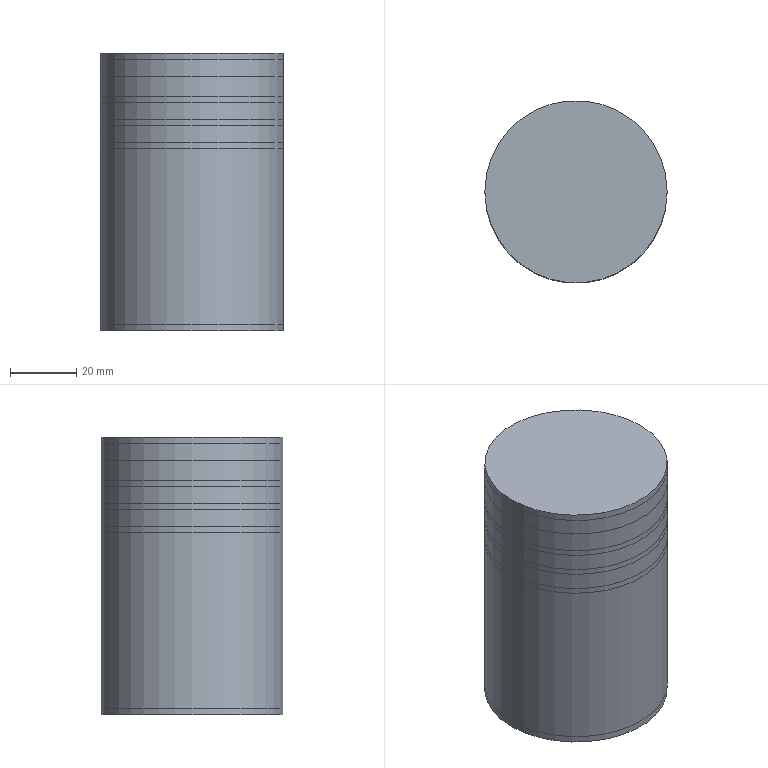Part | NX | features BREP 2 | 2 solids | 27 faces | box 55 x 55 x 83.85 mm | volume 287386 mm3 | plane 11 | cylinder 10 | torus 6 | commonest cylinder face diameters 54.996 x4 52.246 x3 40.002 x1 54.96 x1 55 x1
STEP:
#1=CARTESIAN_POINT('',(27.498,0.,-13.125));
#2=VERTEX_POINT('',#1);
#3=CARTESIAN_POINT('',(0.,0.,-13.125));
#4=DIRECTION('',(0.,0.,1.));
#5=DIRECTION('',(1.,0.,0.));
#6=AXIS2_PLACEMENT_3D('',#3,#4,#5);
#7=CIRCLE('',#6,27.498);
#8=EDGE_CURVE('',#2,#2,#7,.T.);
#9=ORIENTED_EDGE('',*,*,#8,.T.);
#10=EDGE_LOOP('',(#9));
#11=FACE_BOUND('',#10,.T.);
#12=CARTESIAN_POINT('',(27.498,0.,-7.));
#13=VERTEX_POINT('',#12);
#14=CARTESIAN_POINT('',(0.,0.,-7.));
#15=DIRECTION('',(0.,0.,1.));
#16=DIRECTION('',(1.,0.,0.));
#17=AXIS2_PLACEMENT_3D('',#14,#15,#16);
#18=CIRCLE('',#17,27.498);
#19=EDGE_CURVE('',#13,#13,#18,.T.);
#20=ORIENTED_EDGE('',*,*,#19,.F.);
#21=EDGE_LOOP('',(#20));
#22=FACE_BOUND('',#21,.T.);
#23=CARTESIAN_POINT('',(0.,0.,-2.));
#24=DIRECTION('',(0.,0.,-1.));
#25=DIRECTION('',(1.,0.,0.));
#26=AXIS2_PLACEMENT_3D('',#23,#24,#25);
#27=CYLINDRICAL_SURFACE('',#26,27.498);
#28=ADVANCED_FACE('',(#11,#22),#27,.T.);
#29=CARTESIAN_POINT('',(-20.001,0.,-2.));
#30=VERTEX_POINT('',#29);
#31=CARTESIAN_POINT('',(0.,0.,-2.));
#32=DIRECTION('',(0.,0.,-1.));
#33=DIRECTION('',(-1.,0.,0.));
#34=AXIS2_PLACEMENT_3D('',#31,#32,#33);
#35=CIRCLE('',#34,20.001);
#36=EDGE_CURVE('',#30,#30,#35,.T.);
#37=ORIENTED_EDGE('',*,*,#36,.T.);
#38=EDGE_LOOP('',(#37));
#39=FACE_BOUND('',#38,.T.);
#40=CARTESIAN_POINT('',(27.48,0.,-2.));
#41=VERTEX_POINT('',#40);
#42=CARTESIAN_POINT('',(0.,0.,-2.));
#43=DIRECTION('',(0.,0.,1.));
#44=DIRECTION('',(1.,0.,0.));
#45=AXIS2_PLACEMENT_3D('',#42,#43,#44);
#46=CIRCLE('',#45,27.48);
#47=EDGE_CURVE('',#41,#41,#46,.T.);
#48=ORIENTED_EDGE('',*,*,#47,.T.);
#49=EDGE_LOOP('',(#48));
#50=FACE_BOUND('',#49,.T.);
#51=CARTESIAN_POINT('',(0.,0.,-2.));
#52=DIRECTION('',(0.,0.,1.));
#53=DIRECTION('',(-1.,0.,0.));
#54=AXIS2_PLACEMENT_3D('',#51,#52,#53);
#55=PLANE('',#54);
#56=ADVANCED_FACE('',(#39,#50),#55,.T.);
#57=CARTESIAN_POINT('',(27.498,0.,-81.85));
#58=VERTEX_POINT('',#57);
#59=CARTESIAN_POINT('',(0.,0.,-81.85));
#60=DIRECTION('',(0.,0.,1.));
#61=DIRECTION('',(1.,0.,0.));
#62=AXIS2_PLACEMENT_3D('',#59,#60,#61);
#63=CIRCLE('',#62,27.498);
#64=EDGE_CURVE('',#58,#58,#63,.T.);
#65=ORIENTED_EDGE('',*,*,#64,.T.);
#66=EDGE_LOOP('',(#65));
#67=FACE_BOUND('',#66,.T.);
#68=CARTESIAN_POINT('',(27.498,0.,-28.875));
#69=VERTEX_POINT('',#68);
#70=CARTESIAN_POINT('',(0.,0.,-28.875));
#71=DIRECTION('',(0.,0.,1.));
#72=DIRECTION('',(1.,0.,0.));
#73=AXIS2_PLACEMENT_3D('',#70,#71,#72);
#74=CIRCLE('',#73,27.498);
#75=EDGE_CURVE('',#69,#69,#74,.T.);
#76=ORIENTED_EDGE('',*,*,#75,.F.);
#77=EDGE_LOOP('',(#76));
#78=FACE_BOUND('',#77,.T.);
#79=CARTESIAN_POINT('',(0.,0.,-2.));
#80=DIRECTION('',(0.,0.,-1.));
#81=DIRECTION('',(1.,0.,0.));
#82=AXIS2_PLACEMENT_3D('',#79,#80,#81);
#83=CYLINDRICAL_SURFACE('',#82,27.498);
#84=ADVANCED_FACE('',(#67,#78),#83,.T.);
#85=CARTESIAN_POINT('',(27.498,0.,-27.125));
#86=VERTEX_POINT('',#85);
#87=CARTESIAN_POINT('',(0.,0.,-27.125));
#88=DIRECTION('',(0.,0.,1.));
#89=DIRECTION('',(1.,0.,0.));
#90=AXIS2_PLACEMENT_3D('',#87,#88,#89);
#91=CIRCLE('',#90,27.498);
#92=EDGE_CURVE('',#86,#86,#91,.T.);
#93=ORIENTED_EDGE('',*,*,#92,.T.);
#94=EDGE_LOOP('',(#93));
#95=FACE_BOUND('',#94,.T.);
#96=CARTESIAN_POINT('',(27.498,0.,-21.875));
#97=VERTEX_POINT('',#96);
#98=CARTESIAN_POINT('',(0.,0.,-21.875));
#99=DIRECTION('',(0.,0.,1.));
#100=DIRECTION('',(1.,0.,0.));
#101=AXIS2_PLACEMENT_3D('',#98,#99,#100);
#102=CIRCLE('',#101,27.498);
#103=EDGE_CURVE('',#97,#97,#102,.T.);
#104=ORIENTED_EDGE('',*,*,#103,.F.);
#105=EDGE_LOOP('',(#104));
#106=FACE_BOUND('',#105,.T.);
#107=CARTESIAN_POINT('',(0.,0.,-2.));
#108=DIRECTION('',(0.,0.,-1.));
#109=DIRECTION('',(1.,0.,0.));
#110=AXIS2_PLACEMENT_3D('',#107,#108,#109);
#111=CYLINDRICAL_SURFACE('',#110,27.498);
#112=ADVANCED_FACE('',(#95,#106),#111,.T.);
#113=CARTESIAN_POINT('',(27.498,0.,-20.125));
#114=VERTEX_POINT('',#113);
#115=CARTESIAN_POINT('',(0.,0.,-20.125));
#116=DIRECTION('',(0.,0.,1.));
#117=DIRECTION('',(1.,0.,0.));
#118=AXIS2_PLACEMENT_3D('',#115,#116,#117);
#119=CIRCLE('',#118,27.498);
#120=EDGE_CURVE('',#114,#114,#119,.T.);
#121=ORIENTED_EDGE('',*,*,#120,.T.);
#122=EDGE_LOOP('',(#121));
#123=FACE_BOUND('',#122,.T.);
#124=CARTESIAN_POINT('',(27.498,0.,-14.875));
#125=VERTEX_POINT('',#124);
#126=CARTESIAN_POINT('',(0.,0.,-14.875));
#127=DIRECTION('',(0.,0.,1.));
#128=DIRECTION('',(1.,0.,0.));
#129=AXIS2_PLACEMENT_3D('',#126,#127,#128);
#130=CIRCLE('',#129,27.498);
#131=EDGE_CURVE('',#125,#125,#130,.T.);
#132=ORIENTED_EDGE('',*,*,#131,.F.);
#133=EDGE_LOOP('',(#132));
#134=FACE_BOUND('',#133,.T.);
#135=CARTESIAN_POINT('',(0.,0.,-2.));
#136=DIRECTION('',(0.,0.,-1.));
#137=DIRECTION('',(1.,0.,0.));
#138=AXIS2_PLACEMENT_3D('',#135,#136,#137);
#139=CYLINDRICAL_SURFACE('',#138,27.498);
#140=ADVANCED_FACE('',(#123,#134),#139,.T.);
#141=CARTESIAN_POINT('',(-20.001,0.,-81.85));
#142=VERTEX_POINT('',#141);
#143=CARTESIAN_POINT('',(0.,0.,-81.85));
#144=DIRECTION('',(0.,0.,-1.));
#145=DIRECTION('',(-1.,0.,0.));
#146=AXIS2_PLACEMENT_3D('',#143,#144,#145);
#147=CIRCLE('',#146,20.001);
#148=EDGE_CURVE('',#142,#142,#147,.T.);
#149=ORIENTED_EDGE('',*,*,#148,.F.);
#150=EDGE_LOOP('',(#149));
#151=FACE_BOUND('',#150,.T.);
#152=ORIENTED_EDGE('',*,*,#64,.F.);
#153=EDGE_LOOP('',(#152));
#154=FACE_BOUND('',#153,.T.);
#155=CARTESIAN_POINT('',(0.,0.,-81.85));
#156=DIRECTION('',(0.,0.,1.));
#157=DIRECTION('',(-1.,0.,0.));
#158=AXIS2_PLACEMENT_3D('',#155,#156,#157);
#159=PLANE('',#158);
#160=ADVANCED_FACE('',(#151,#154),#159,.F.);
#161=ORIENTED_EDGE('',*,*,#148,.T.);
#162=EDGE_LOOP('',(#161));
#163=FACE_BOUND('',#162,.T.);
#164=ORIENTED_EDGE('',*,*,#36,.F.);
#165=EDGE_LOOP('',(#164));
#166=FACE_BOUND('',#165,.T.);
#167=CARTESIAN_POINT('',(0.,0.,-2.));
#168=DIRECTION('',(0.,0.,-1.));
#169=DIRECTION('',(1.,0.,0.));
#170=AXIS2_PLACEMENT_3D('',#167,#168,#169);
#171=CYLINDRICAL_SURFACE('',#170,20.001);
#172=ADVANCED_FACE('',(#163,#166),#171,.F.);
#173=CARTESIAN_POINT('',(26.723,0.,-14.875));
#174=VERTEX_POINT('',#173);
#175=CARTESIAN_POINT('',(0.,0.,-14.875));
#176=DIRECTION('',(0.,0.,1.));
#177=DIRECTION('',(1.,0.,0.));
#178=AXIS2_PLACEMENT_3D('',#175,#176,#177);
#179=CIRCLE('',#178,26.723);
#180=EDGE_CURVE('',#174,#174,#179,.T.);
#181=ORIENTED_EDGE('',*,*,#180,.F.);
#182=EDGE_LOOP('',(#181));
#183=FACE_BOUND('',#182,.T.);
#184=ORIENTED_EDGE('',*,*,#131,.T.);
#185=EDGE_LOOP('',(#184));
#186=FACE_BOUND('',#185,.T.);
#187=CARTESIAN_POINT('',(0.,0.,-14.875));
#188=DIRECTION('',(0.,0.,1.));
#189=DIRECTION('',(-1.,0.,0.));
#190=AXIS2_PLACEMENT_3D('',#187,#188,#189);
#191=PLANE('',#190);
#192=ADVANCED_FACE('',(#183,#186),#191,.T.);
#193=CARTESIAN_POINT('',(26.723,0.,-13.125));
#194=VERTEX_POINT('',#193);
#195=CARTESIAN_POINT('',(0.,0.,-13.125));
#196=DIRECTION('',(0.,0.,1.));
#197=DIRECTION('',(1.,0.,0.));
#198=AXIS2_PLACEMENT_3D('',#195,#196,#197);
#199=CIRCLE('',#198,26.723);
#200=EDGE_CURVE('',#194,#194,#199,.T.);
#201=ORIENTED_EDGE('',*,*,#200,.T.);
#202=EDGE_LOOP('',(#201));
#203=FACE_BOUND('',#202,.T.);
#204=ORIENTED_EDGE('',*,*,#8,.F.);
#205=EDGE_LOOP('',(#204));
#206=FACE_BOUND('',#205,.T.);
#207=CARTESIAN_POINT('',(0.,0.,-13.125));
#208=DIRECTION('',(0.,0.,1.));
#209=DIRECTION('',(-1.,0.,0.));
#210=AXIS2_PLACEMENT_3D('',#207,#208,#209);
#211=PLANE('',#210);
#212=ADVANCED_FACE('',(#203,#206),#211,.F.);
#213=CARTESIAN_POINT('',(26.123,0.,-13.725));
#214=VERTEX_POINT('',#213);
#215=CARTESIAN_POINT('',(0.,0.,-13.725));
#216=DIRECTION('',(0.,0.,1.));
#217=DIRECTION('',(1.,0.,0.));
#218=AXIS2_PLACEMENT_3D('',#215,#216,#217);
#219=CIRCLE('',#218,26.123);
#220=EDGE_CURVE('',#214,#214,#219,.T.);
#221=ORIENTED_EDGE('',*,*,#220,.F.);
#222=EDGE_LOOP('',(#221));
#223=FACE_BOUND('',#222,.T.);
#224=CARTESIAN_POINT('',(26.123,0.,-14.275));
#225=VERTEX_POINT('',#224);
#226=CARTESIAN_POINT('',(0.,0.,-14.275));
#227=DIRECTION('',(0.,0.,1.));
#228=DIRECTION('',(1.,0.,0.));
#229=AXIS2_PLACEMENT_3D('',#226,#227,#228);
#230=CIRCLE('',#229,26.123);
#231=EDGE_CURVE('',#225,#225,#230,.T.);
#232=ORIENTED_EDGE('',*,*,#231,.T.);
#233=EDGE_LOOP('',(#232));
#234=FACE_BOUND('',#233,.T.);
#235=CARTESIAN_POINT('',(0.,0.,-14.));
#236=DIRECTION('',(0.,0.,1.));
#237=DIRECTION('',(-1.,0.,0.));
#238=AXIS2_PLACEMENT_3D('',#235,#236,#237);
#239=CYLINDRICAL_SURFACE('',#238,26.123);
#240=ADVANCED_FACE('',(#223,#234),#239,.T.);
#241=ORIENTED_EDGE('',*,*,#180,.T.);
#242=EDGE_LOOP('',(#241));
#243=FACE_BOUND('',#242,.T.);
#244=ORIENTED_EDGE('',*,*,#231,.F.);
#245=EDGE_LOOP('',(#244));
#246=FACE_BOUND('',#245,.T.);
#247=CARTESIAN_POINT('',(0.,0.,-14.275));
#248=DIRECTION('',(0.,0.,1.));
#249=DIRECTION('',(-1.,0.,0.));
#250=AXIS2_PLACEMENT_3D('',#247,#248,#249);
#251=TOROIDAL_SURFACE('',#250,26.723,0.6);
#252=ADVANCED_FACE('',(#243,#246),#251,.F.);
#253=ORIENTED_EDGE('',*,*,#200,.F.);
#254=EDGE_LOOP('',(#253));
#255=FACE_BOUND('',#254,.T.);
#256=ORIENTED_EDGE('',*,*,#220,.T.);
#257=EDGE_LOOP('',(#256));
#258=FACE_BOUND('',#257,.T.);
#259=CARTESIAN_POINT('',(0.,0.,-13.725));
#260=DIRECTION('',(0.,0.,1.));
#261=DIRECTION('',(-1.,0.,0.));
#262=AXIS2_PLACEMENT_3D('',#259,#260,#261);
#263=TOROIDAL_SURFACE('',#262,26.723,0.6);
#264=ADVANCED_FACE('',(#255,#258),#263,.F.);
#265=CARTESIAN_POINT('',(26.723,0.,-20.125));
#266=VERTEX_POINT('',#265);
#267=CARTESIAN_POINT('',(0.,0.,-20.125));
#268=DIRECTION('',(0.,0.,1.));
#269=DIRECTION('',(1.,0.,0.));
#270=AXIS2_PLACEMENT_3D('',#267,#268,#269);
#271=CIRCLE('',#270,26.723);
#272=EDGE_CURVE('',#266,#266,#271,.T.);
#273=ORIENTED_EDGE('',*,*,#272,.T.);
#274=EDGE_LOOP('',(#273));
#275=FACE_BOUND('',#274,.T.);
#276=ORIENTED_EDGE('',*,*,#120,.F.);
#277=EDGE_LOOP('',(#276));
#278=FACE_BOUND('',#277,.T.);
#279=CARTESIAN_POINT('',(0.,0.,-20.125));
#280=DIRECTION('',(0.,0.,1.));
#281=DIRECTION('',(-1.,0.,0.));
#282=AXIS2_PLACEMENT_3D('',#279,#280,#281);
#283=PLANE('',#282);
#284=ADVANCED_FACE('',(#275,#278),#283,.F.);
#285=CARTESIAN_POINT('',(26.723,0.,-21.875));
#286=VERTEX_POINT('',#285);
#287=CARTESIAN_POINT('',(0.,0.,-21.875));
#288=DIRECTION('',(0.,0.,1.));
#289=DIRECTION('',(1.,0.,0.));
#290=AXIS2_PLACEMENT_3D('',#287,#288,#289);
#291=CIRCLE('',#290,26.723);
#292=EDGE_CURVE('',#286,#286,#291,.T.);
#293=ORIENTED_EDGE('',*,*,#292,.F.);
#294=EDGE_LOOP('',(#293));
#295=FACE_BOUND('',#294,.T.);
#296=ORIENTED_EDGE('',*,*,#103,.T.);
#297=EDGE_LOOP('',(#296));
#298=FACE_BOUND('',#297,.T.);
#299=CARTESIAN_POINT('',(0.,0.,-21.875));
#300=DIRECTION('',(0.,0.,1.));
#301=DIRECTION('',(-1.,0.,0.));
#302=AXIS2_PLACEMENT_3D('',#299,#300,#301);
#303=PLANE('',#302);
#304=ADVANCED_FACE('',(#295,#298),#303,.T.);
#305=CARTESIAN_POINT('',(26.123,0.,-20.725));
#306=VERTEX_POINT('',#305);
#307=CARTESIAN_POINT('',(0.,0.,-20.725));
#308=DIRECTION('',(0.,0.,1.));
#309=DIRECTION('',(1.,0.,0.));
#310=AXIS2_PLACEMENT_3D('',#307,#308,#309);
#311=CIRCLE('',#310,26.123);
#312=EDGE_CURVE('',#306,#306,#311,.T.);
#313=ORIENTED_EDGE('',*,*,#312,.F.);
#314=EDGE_LOOP('',(#313));
#315=FACE_BOUND('',#314,.T.);
#316=CARTESIAN_POINT('',(26.123,0.,-21.275));
#317=VERTEX_POINT('',#316);
#318=CARTESIAN_POINT('',(0.,0.,-21.275));
#319=DIRECTION('',(0.,0.,1.));
#320=DIRECTION('',(1.,0.,0.));
#321=AXIS2_PLACEMENT_3D('',#318,#319,#320);
#322=CIRCLE('',#321,26.123);
#323=EDGE_CURVE('',#317,#317,#322,.T.);
#324=ORIENTED_EDGE('',*,*,#323,.T.);
#325=EDGE_LOOP('',(#324));
#326=FACE_BOUND('',#325,.T.);
#327=CARTESIAN_POINT('',(0.,0.,-21.));
#328=DIRECTION('',(0.,0.,1.));
#329=DIRECTION('',(-1.,0.,0.));
#330=AXIS2_PLACEMENT_3D('',#327,#328,#329);
#331=CYLINDRICAL_SURFACE('',#330,26.123);
#332=ADVANCED_FACE('',(#315,#326),#331,.T.);
#333=ORIENTED_EDGE('',*,*,#292,.T.);
#334=EDGE_LOOP('',(#333));
#335=FACE_BOUND('',#334,.T.);
#336=ORIENTED_EDGE('',*,*,#323,.F.);
#337=EDGE_LOOP('',(#336));
#338=FACE_BOUND('',#337,.T.);
#339=CARTESIAN_POINT('',(0.,0.,-21.275));
#340=DIRECTION('',(0.,0.,1.));
#341=DIRECTION('',(-1.,0.,0.));
#342=AXIS2_PLACEMENT_3D('',#339,#340,#341);
#343=TOROIDAL_SURFACE('',#342,26.723,0.6);
#344=ADVANCED_FACE('',(#335,#338),#343,.F.);
#345=ORIENTED_EDGE('',*,*,#272,.F.);
#346=EDGE_LOOP('',(#345));
#347=FACE_BOUND('',#346,.T.);
#348=ORIENTED_EDGE('',*,*,#312,.T.);
#349=EDGE_LOOP('',(#348));
#350=FACE_BOUND('',#349,.T.);
#351=CARTESIAN_POINT('',(0.,0.,-20.725));
#352=DIRECTION('',(0.,0.,1.));
#353=DIRECTION('',(-1.,0.,0.));
#354=AXIS2_PLACEMENT_3D('',#351,#352,#353);
#355=TOROIDAL_SURFACE('',#354,26.723,0.6);
#356=ADVANCED_FACE('',(#347,#350),#355,.F.);
#357=CARTESIAN_POINT('',(26.723,0.,-27.125));
#358=VERTEX_POINT('',#357);
#359=CARTESIAN_POINT('',(0.,0.,-27.125));
#360=DIRECTION('',(0.,0.,1.));
#361=DIRECTION('',(1.,0.,0.));
#362=AXIS2_PLACEMENT_3D('',#359,#360,#361);
#363=CIRCLE('',#362,26.723);
#364=EDGE_CURVE('',#358,#358,#363,.T.);
#365=ORIENTED_EDGE('',*,*,#364,.T.);
#366=EDGE_LOOP('',(#365));
#367=FACE_BOUND('',#366,.T.);
#368=ORIENTED_EDGE('',*,*,#92,.F.);
#369=EDGE_LOOP('',(#368));
#370=FACE_BOUND('',#369,.T.);
#371=CARTESIAN_POINT('',(0.,0.,-27.125));
#372=DIRECTION('',(0.,0.,1.));
#373=DIRECTION('',(-1.,0.,0.));
#374=AXIS2_PLACEMENT_3D('',#371,#372,#373);
#375=PLANE('',#374);
#376=ADVANCED_FACE('',(#367,#370),#375,.F.);
#377=CARTESIAN_POINT('',(26.723,0.,-28.875));
#378=VERTEX_POINT('',#377);
#379=CARTESIAN_POINT('',(0.,0.,-28.875));
#380=DIRECTION('',(0.,0.,1.));
#381=DIRECTION('',(1.,0.,0.));
#382=AXIS2_PLACEMENT_3D('',#379,#380,#381);
#383=CIRCLE('',#382,26.723);
#384=EDGE_CURVE('',#378,#378,#383,.T.);
#385=ORIENTED_EDGE('',*,*,#384,.F.);
#386=EDGE_LOOP('',(#385));
#387=FACE_BOUND('',#386,.T.);
#388=ORIENTED_EDGE('',*,*,#75,.T.);
#389=EDGE_LOOP('',(#388));
#390=FACE_BOUND('',#389,.T.);
#391=CARTESIAN_POINT('',(0.,0.,-28.875));
#392=DIRECTION('',(0.,0.,1.));
#393=DIRECTION('',(-1.,0.,0.));
#394=AXIS2_PLACEMENT_3D('',#391,#392,#393);
#395=PLANE('',#394);
#396=ADVANCED_FACE('',(#387,#390),#395,.T.);
#397=CARTESIAN_POINT('',(26.123,0.,-27.725));
#398=VERTEX_POINT('',#397);
#399=CARTESIAN_POINT('',(0.,0.,-27.725));
#400=DIRECTION('',(0.,0.,1.));
#401=DIRECTION('',(1.,0.,0.));
#402=AXIS2_PLACEMENT_3D('',#399,#400,#401);
#403=CIRCLE('',#402,26.123);
#404=EDGE_CURVE('',#398,#398,#403,.T.);
#405=ORIENTED_EDGE('',*,*,#404,.F.);
#406=EDGE_LOOP('',(#405));
#407=FACE_BOUND('',#406,.T.);
#408=CARTESIAN_POINT('',(26.123,0.,-28.275));
#409=VERTEX_POINT('',#408);
#410=CARTESIAN_POINT('',(0.,0.,-28.275));
#411=DIRECTION('',(0.,0.,1.));
#412=DIRECTION('',(1.,0.,0.));
#413=AXIS2_PLACEMENT_3D('',#410,#411,#412);
#414=CIRCLE('',#413,26.123);
#415=EDGE_CURVE('',#409,#409,#414,.T.);
#416=ORIENTED_EDGE('',*,*,#415,.T.);
#417=EDGE_LOOP('',(#416));
#418=FACE_BOUND('',#417,.T.);
#419=CARTESIAN_POINT('',(0.,0.,-28.));
#420=DIRECTION('',(0.,0.,1.));
#421=DIRECTION('',(-1.,0.,0.));
#422=AXIS2_PLACEMENT_3D('',#419,#420,#421);
#423=CYLINDRICAL_SURFACE('',#422,26.123);
#424=ADVANCED_FACE('',(#407,#418),#423,.T.);
#425=ORIENTED_EDGE('',*,*,#384,.T.);
#426=EDGE_LOOP('',(#425));
#427=FACE_BOUND('',#426,.T.);
#428=ORIENTED_EDGE('',*,*,#415,.F.);
#429=EDGE_LOOP('',(#428));
#430=FACE_BOUND('',#429,.T.);
#431=CARTESIAN_POINT('',(0.,0.,-28.275));
#432=DIRECTION('',(0.,0.,1.));
#433=DIRECTION('',(-1.,0.,0.));
#434=AXIS2_PLACEMENT_3D('',#431,#432,#433);
#435=TOROIDAL_SURFACE('',#434,26.723,0.6);
#436=ADVANCED_FACE('',(#427,#430),#435,.F.);
#437=ORIENTED_EDGE('',*,*,#364,.F.);
#438=EDGE_LOOP('',(#437));
#439=FACE_BOUND('',#438,.T.);
#440=ORIENTED_EDGE('',*,*,#404,.T.);
#441=EDGE_LOOP('',(#440));
#442=FACE_BOUND('',#441,.T.);
#443=CARTESIAN_POINT('',(0.,0.,-27.725));
#444=DIRECTION('',(0.,0.,1.));
#445=DIRECTION('',(-1.,0.,0.));
#446=AXIS2_PLACEMENT_3D('',#443,#444,#445);
#447=TOROIDAL_SURFACE('',#446,26.723,0.6);
#448=ADVANCED_FACE('',(#439,#442),#447,.F.);
#449=CARTESIAN_POINT('',(27.48,0.,-7.));
#450=VERTEX_POINT('',#449);
#451=CARTESIAN_POINT('',(0.,0.,-7.));
#452=DIRECTION('',(0.,0.,1.));
#453=DIRECTION('',(1.,0.,0.));
#454=AXIS2_PLACEMENT_3D('',#451,#452,#453);
#455=CIRCLE('',#454,27.48);
#456=EDGE_CURVE('',#450,#450,#455,.T.);
#457=ORIENTED_EDGE('',*,*,#456,.F.);
#458=EDGE_LOOP('',(#457));
#459=FACE_BOUND('',#458,.T.);
#460=ORIENTED_EDGE('',*,*,#19,.T.);
#461=EDGE_LOOP('',(#460));
#462=FACE_BOUND('',#461,.T.);
#463=CARTESIAN_POINT('',(0.,0.,-7.));
#464=DIRECTION('',(0.,0.,1.));
#465=DIRECTION('',(-1.,0.,0.));
#466=AXIS2_PLACEMENT_3D('',#463,#464,#465);
#467=PLANE('',#466);
#468=ADVANCED_FACE('',(#459,#462),#467,.T.);
#469=ORIENTED_EDGE('',*,*,#47,.F.);
#470=EDGE_LOOP('',(#469));
#471=FACE_BOUND('',#470,.T.);
#472=ORIENTED_EDGE('',*,*,#456,.T.);
#473=EDGE_LOOP('',(#472));
#474=FACE_BOUND('',#473,.T.);
#475=CARTESIAN_POINT('',(0.,0.,-4.5));
#476=DIRECTION('',(0.,0.,1.));
#477=DIRECTION('',(-1.,0.,0.));
#478=AXIS2_PLACEMENT_3D('',#475,#476,#477);
#479=CYLINDRICAL_SURFACE('',#478,27.48);
#480=ADVANCED_FACE('',(#471,#474),#479,.T.);
#481=CLOSED_SHELL('',(#28,#56,#84,#112,#140,#160,#172,#192,#212,#240,#252,#264,#284,#304,#332,#344,#356,#376,#396,#424,#436,#448,#468,#480));
#482=MANIFOLD_SOLID_BREP('',#481);
#483=CARTESIAN_POINT('',(27.5,0.,0.));
#484=VERTEX_POINT('',#483);
#485=CARTESIAN_POINT('',(0.,0.,0.));
#486=DIRECTION('',(0.,0.,1.));
#487=DIRECTION('',(1.,0.,0.));
#488=AXIS2_PLACEMENT_3D('',#485,#486,#487);
#489=CIRCLE('',#488,27.5);
#490=EDGE_CURVE('',#484,#484,#489,.T.);
#491=ORIENTED_EDGE('',*,*,#490,.F.);
#492=EDGE_LOOP('',(#491));
#493=FACE_BOUND('',#492,.T.);
#494=CARTESIAN_POINT('',(27.5,0.,-83.85));
#495=VERTEX_POINT('',#494);
#496=CARTESIAN_POINT('',(0.,0.,-83.85));
#497=DIRECTION('',(0.,0.,1.));
#498=DIRECTION('',(1.,0.,0.));
#499=AXIS2_PLACEMENT_3D('',#496,#497,#498);
#500=CIRCLE('',#499,27.5);
#501=EDGE_CURVE('',#495,#495,#500,.T.);
#502=ORIENTED_EDGE('',*,*,#501,.T.);
#503=EDGE_LOOP('',(#502));
#504=FACE_BOUND('',#503,.T.);
#505=CARTESIAN_POINT('',(0.,0.,0.));
#506=DIRECTION('',(0.,0.,-1.));
#507=DIRECTION('',(1.,0.,0.));
#508=AXIS2_PLACEMENT_3D('',#505,#506,#507);
#509=CYLINDRICAL_SURFACE('',#508,27.5);
#510=ADVANCED_FACE('',(#493,#504),#509,.T.);
#511=ORIENTED_EDGE('',*,*,#490,.T.);
#512=EDGE_LOOP('',(#511));
#513=FACE_BOUND('',#512,.T.);
#514=CARTESIAN_POINT('',(0.,0.,0.));
#515=DIRECTION('',(0.,0.,1.));
#516=DIRECTION('',(-1.,0.,0.));
#517=AXIS2_PLACEMENT_3D('',#514,#515,#516);
#518=PLANE('',#517);
#519=ADVANCED_FACE('',(#513),#518,.T.);
#520=ORIENTED_EDGE('',*,*,#501,.F.);
#521=EDGE_LOOP('',(#520));
#522=FACE_BOUND('',#521,.T.);
#523=CARTESIAN_POINT('',(0.,0.,-83.85));
#524=DIRECTION('',(0.,0.,1.));
#525=DIRECTION('',(-1.,0.,0.));
#526=AXIS2_PLACEMENT_3D('',#523,#524,#525);
#527=PLANE('',#526);
#528=ADVANCED_FACE('',(#522),#527,.F.);
#529=CLOSED_SHELL('',(#510,#519,#528));
#530=MANIFOLD_SOLID_BREP('',#529);
#531=(LENGTH_UNIT()NAMED_UNIT(*)SI_UNIT(.MILLI.,.METRE.));
#532=UNCERTAINTY_MEASURE_WITH_UNIT(LENGTH_MEASURE(0.00001),#531,'','');
#533=(NAMED_UNIT(*)PLANE_ANGLE_UNIT()SI_UNIT($,.RADIAN.));
#534=(NAMED_UNIT(*)SI_UNIT($,.STERADIAN.)SOLID_ANGLE_UNIT());
#535=(GEOMETRIC_REPRESENTATION_CONTEXT(3)GLOBAL_UNCERTAINTY_ASSIGNED_CONTEXT((#532))GLOBAL_UNIT_ASSIGNED_CONTEXT((#531,#533,#534))REPRESENTATION_CONTEXT('',''));
#536=ADVANCED_BREP_SHAPE_REPRESENTATION('',(#482,#530),#535);